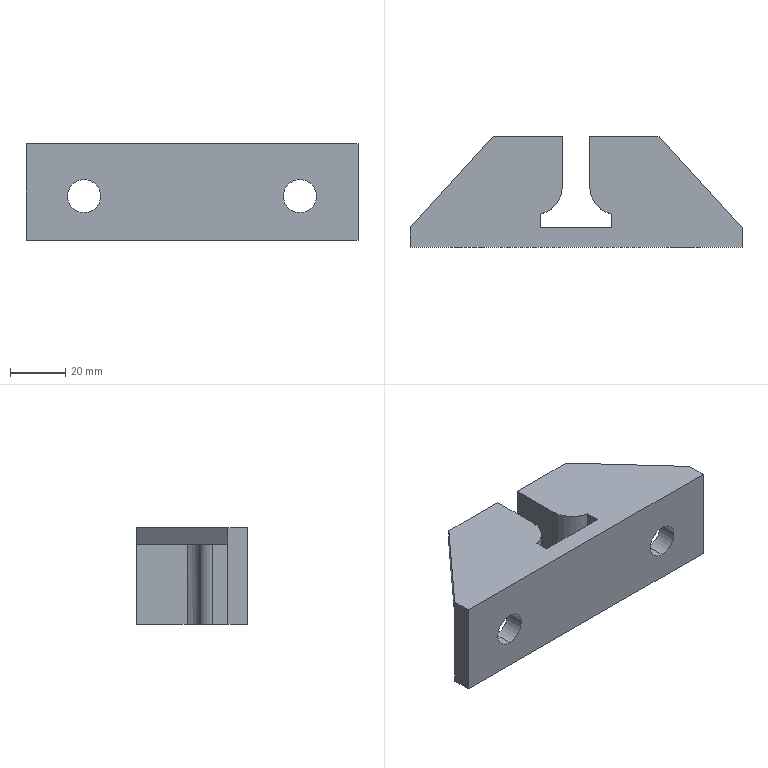Part | SolidWorks | features ICE 3, Fillet 2, MirrorPattern 2, Extrusion 1 | 1 solid | 32 faces | box 120 x 40 x 35 mm | volume 52086 mm3 | plane 22 | cylinder 8 | spline 2 | commonest cylinder face diameters 12 x4 10 x2 20 x2
STEP:
#1=CARTESIAN_POINT('',(39.,0.,-4.638));
#2=VERTEX_POINT('',#1);
#3=CARTESIAN_POINT('',(39.,0.,-16.638));
#4=VERTEX_POINT('',#3);
#5=CARTESIAN_POINT('',(39.,0.,-10.638));
#6=DIRECTION('',(0.,-1.,0.));
#7=DIRECTION('',(0.,0.,1.));
#8=AXIS2_PLACEMENT_3D('',#5,#6,#7);
#9=CIRCLE('',#8,6.);
#10=EDGE_CURVE('',#2,#4,#9,.T.);
#11=ORIENTED_EDGE('',*,*,#10,.T.);
#12=CARTESIAN_POINT('',(39.,7.,-16.638));
#13=VERTEX_POINT('',#12);
#14=CARTESIAN_POINT('',(39.,-3.,-16.638));
#15=DIRECTION('',(0.,1.,0.));
#16=VECTOR('',#15,1000.);
#17=LINE('',#14,#16);
#18=EDGE_CURVE('',#4,#13,#17,.T.);
#19=ORIENTED_EDGE('',*,*,#18,.T.);
#20=CARTESIAN_POINT('',(39.,7.,-4.638));
#21=VERTEX_POINT('',#20);
#22=CARTESIAN_POINT('',(39.,7.,-10.638));
#23=DIRECTION('',(0.,-1.,0.));
#24=DIRECTION('',(0.,0.,1.));
#25=AXIS2_PLACEMENT_3D('',#22,#23,#24);
#26=CIRCLE('',#25,6.);
#27=EDGE_CURVE('',#21,#13,#26,.T.);
#28=ORIENTED_EDGE('',*,*,#27,.F.);
#29=CARTESIAN_POINT('',(39.,-3.,-4.638));
#30=DIRECTION('',(0.,1.,0.));
#31=VECTOR('',#30,1000.);
#32=LINE('',#29,#31);
#33=EDGE_CURVE('',#2,#21,#32,.T.);
#34=ORIENTED_EDGE('',*,*,#33,.F.);
#35=EDGE_LOOP('',(#11,#19,#28,#34));
#36=FACE_OUTER_BOUND('',#35,.T.);
#37=CARTESIAN_POINT('',(39.,-3.,-10.638));
#38=DIRECTION('',(0.,1.,0.));
#39=DIRECTION('',(0.,0.,1.));
#40=AXIS2_PLACEMENT_3D('',#37,#38,#39);
#41=CYLINDRICAL_SURFACE('',#40,6.);
#42=ADVANCED_FACE('',(#36),#41,.F.);
#43=CARTESIAN_POINT('',(-39.,0.,-16.638));
#44=VERTEX_POINT('',#43);
#45=CARTESIAN_POINT('',(-39.,0.,-4.638));
#46=VERTEX_POINT('',#45);
#47=CARTESIAN_POINT('',(-39.,0.,-10.638));
#48=DIRECTION('',(0.,1.,0.));
#49=DIRECTION('',(0.,0.,1.));
#50=AXIS2_PLACEMENT_3D('',#47,#48,#49);
#51=CIRCLE('',#50,6.);
#52=EDGE_CURVE('',#44,#46,#51,.T.);
#53=ORIENTED_EDGE('',*,*,#52,.F.);
#54=CARTESIAN_POINT('',(-39.,7.,-16.638));
#55=VERTEX_POINT('',#54);
#56=CARTESIAN_POINT('',(-39.,-3.,-16.638));
#57=DIRECTION('',(0.,1.,0.));
#58=VECTOR('',#57,1000.);
#59=LINE('',#56,#58);
#60=EDGE_CURVE('',#44,#55,#59,.T.);
#61=ORIENTED_EDGE('',*,*,#60,.T.);
#62=CARTESIAN_POINT('',(-39.,7.,-4.638));
#63=VERTEX_POINT('',#62);
#64=CARTESIAN_POINT('',(-39.,7.,-10.638));
#65=DIRECTION('',(0.,1.,0.));
#66=DIRECTION('',(0.,0.,1.));
#67=AXIS2_PLACEMENT_3D('',#64,#65,#66);
#68=CIRCLE('',#67,6.);
#69=EDGE_CURVE('',#55,#63,#68,.T.);
#70=ORIENTED_EDGE('',*,*,#69,.T.);
#71=CARTESIAN_POINT('',(-39.,-3.,-4.638));
#72=DIRECTION('',(0.,1.,0.));
#73=VECTOR('',#72,1000.);
#74=LINE('',#71,#73);
#75=EDGE_CURVE('',#46,#63,#74,.T.);
#76=ORIENTED_EDGE('',*,*,#75,.F.);
#77=EDGE_LOOP('',(#53,#61,#70,#76));
#78=FACE_OUTER_BOUND('',#77,.T.);
#79=CARTESIAN_POINT('',(-39.,-3.,-10.638));
#80=DIRECTION('',(0.,1.,0.));
#81=DIRECTION('',(0.,0.,1.));
#82=AXIS2_PLACEMENT_3D('',#79,#80,#81);
#83=CYLINDRICAL_SURFACE('',#82,6.);
#84=ADVANCED_FACE('',(#78),#83,.F.);
#85=CARTESIAN_POINT('',(17.,7.,-26.638));
#86=VERTEX_POINT('',#85);
#87=CARTESIAN_POINT('',(17.,7.,2.362));
#88=VERTEX_POINT('',#87);
#89=CARTESIAN_POINT('',(17.,7.,-61.752));
#90=DIRECTION('',(0.,0.,1.));
#91=VECTOR('',#90,1000.);
#92=LINE('',#89,#91);
#93=EDGE_CURVE('',#86,#88,#92,.T.);
#94=ORIENTED_EDGE('',*,*,#93,.T.);
#95=CARTESIAN_POINT('',(60.,7.,2.362));
#96=VERTEX_POINT('',#95);
#97=CARTESIAN_POINT('',(13.,7.,2.362));
#98=DIRECTION('',(-1.,0.,0.));
#99=VECTOR('',#98,1000.);
#100=LINE('',#97,#99);
#101=EDGE_CURVE('',#96,#88,#100,.T.);
#102=ORIENTED_EDGE('',*,*,#101,.F.);
#103=CARTESIAN_POINT('',(60.,7.,-26.638));
#104=VERTEX_POINT('',#103);
#105=CARTESIAN_POINT('',(60.,7.,-26.638));
#106=DIRECTION('',(0.,0.,-1.));
#107=VECTOR('',#106,1000.);
#108=LINE('',#105,#107);
#109=EDGE_CURVE('',#96,#104,#108,.T.);
#110=ORIENTED_EDGE('',*,*,#109,.T.);
#111=CARTESIAN_POINT('',(-60.,7.,-26.638));
#112=DIRECTION('',(-1.,0.,0.));
#113=VECTOR('',#112,1000.);
#114=LINE('',#111,#113);
#115=EDGE_CURVE('',#104,#86,#114,.T.);
#116=ORIENTED_EDGE('',*,*,#115,.T.);
#117=EDGE_LOOP('',(#94,#102,#110,#116));
#118=FACE_OUTER_BOUND('',#117,.T.);
#119=ORIENTED_EDGE('',*,*,#27,.T.);
#120=CARTESIAN_POINT('',(39.,7.,-10.638));
#121=DIRECTION('',(0.,-1.,0.));
#122=DIRECTION('',(0.,0.,1.));
#123=AXIS2_PLACEMENT_3D('',#120,#121,#122);
#124=CIRCLE('',#123,6.);
#125=EDGE_CURVE('',#13,#21,#124,.T.);
#126=ORIENTED_EDGE('',*,*,#125,.T.);
#127=EDGE_LOOP('',(#119,#126));
#128=FACE_BOUND('',#127,.T.);
#129=CARTESIAN_POINT('',(0.,7.,0.));
#130=DIRECTION('',(0.,1.,0.));
#131=DIRECTION('',(0.,0.,1.));
#132=AXIS2_PLACEMENT_3D('',#129,#130,#131);
#133=PLANE('',#132);
#134=ADVANCED_FACE('',(#118,#128),#133,.T.);
#135=CARTESIAN_POINT('',(-60.,0.,-26.638));
#136=VERTEX_POINT('',#135);
#137=CARTESIAN_POINT('',(-60.,0.,8.362));
#138=VERTEX_POINT('',#137);
#139=CARTESIAN_POINT('',(-60.,0.,-26.638));
#140=DIRECTION('',(0.,0.,1.));
#141=VECTOR('',#140,1000.);
#142=LINE('',#139,#141);
#143=EDGE_CURVE('',#136,#138,#142,.T.);
#144=ORIENTED_EDGE('',*,*,#143,.F.);
#145=CARTESIAN_POINT('',(60.,0.,-26.638));
#146=VERTEX_POINT('',#145);
#147=CARTESIAN_POINT('',(-60.,0.,-26.638));
#148=DIRECTION('',(-1.,0.,0.));
#149=VECTOR('',#148,1000.);
#150=LINE('',#147,#149);
#151=EDGE_CURVE('',#146,#136,#150,.T.);
#152=ORIENTED_EDGE('',*,*,#151,.F.);
#153=CARTESIAN_POINT('',(60.,0.,8.362));
#154=VERTEX_POINT('',#153);
#155=CARTESIAN_POINT('',(60.,0.,-26.638));
#156=DIRECTION('',(0.,0.,-1.));
#157=VECTOR('',#156,1000.);
#158=LINE('',#155,#157);
#159=EDGE_CURVE('',#154,#146,#158,.T.);
#160=ORIENTED_EDGE('',*,*,#159,.F.);
#161=CARTESIAN_POINT('',(-60.,0.,8.362));
#162=DIRECTION('',(1.,0.,0.));
#163=VECTOR('',#162,1000.);
#164=LINE('',#161,#163);
#165=EDGE_CURVE('',#138,#154,#164,.T.);
#166=ORIENTED_EDGE('',*,*,#165,.F.);
#167=EDGE_LOOP('',(#144,#152,#160,#166));
#168=FACE_OUTER_BOUND('',#167,.T.);
#169=CARTESIAN_POINT('',(-39.,0.,-10.638));
#170=DIRECTION('',(0.,1.,0.));
#171=DIRECTION('',(0.,0.,1.));
#172=AXIS2_PLACEMENT_3D('',#169,#170,#171);
#173=CIRCLE('',#172,6.);
#174=EDGE_CURVE('',#46,#44,#173,.T.);
#175=ORIENTED_EDGE('',*,*,#174,.T.);
#176=ORIENTED_EDGE('',*,*,#52,.T.);
#177=EDGE_LOOP('',(#175,#176));
#178=FACE_BOUND('',#177,.T.);
#179=ORIENTED_EDGE('',*,*,#10,.F.);
#180=CARTESIAN_POINT('',(39.,0.,-10.638));
#181=DIRECTION('',(0.,-1.,0.));
#182=DIRECTION('',(0.,0.,1.));
#183=AXIS2_PLACEMENT_3D('',#180,#181,#182);
#184=CIRCLE('',#183,6.);
#185=EDGE_CURVE('',#4,#2,#184,.T.);
#186=ORIENTED_EDGE('',*,*,#185,.F.);
#187=EDGE_LOOP('',(#179,#186));
#188=FACE_BOUND('',#187,.T.);
#189=CARTESIAN_POINT('',(0.,0.,0.));
#190=DIRECTION('',(0.,1.,0.));
#191=DIRECTION('',(0.,0.,1.));
#192=AXIS2_PLACEMENT_3D('',#189,#190,#191);
#193=PLANE('',#192);
#194=ADVANCED_FACE('',(#168,#178,#188),#193,.F.);
#195=CARTESIAN_POINT('',(13.,7.,-26.638));
#196=VERTEX_POINT('',#195);
#197=CARTESIAN_POINT('',(13.,7.,8.362));
#198=VERTEX_POINT('',#197);
#199=CARTESIAN_POINT('',(13.,7.,2.362));
#200=DIRECTION('',(0.,0.,1.));
#201=VECTOR('',#200,1000.);
#202=LINE('',#199,#201);
#203=EDGE_CURVE('',#196,#198,#202,.T.);
#204=ORIENTED_EDGE('',*,*,#203,.F.);
#205=CARTESIAN_POINT('',(-13.,7.,-26.638));
#206=VERTEX_POINT('',#205);
#207=CARTESIAN_POINT('',(-60.,7.,-26.638));
#208=DIRECTION('',(-1.,0.,0.));
#209=VECTOR('',#208,1000.);
#210=LINE('',#207,#209);
#211=EDGE_CURVE('',#196,#206,#210,.T.);
#212=ORIENTED_EDGE('',*,*,#211,.T.);
#213=CARTESIAN_POINT('',(-13.,7.,8.362));
#214=VERTEX_POINT('',#213);
#215=CARTESIAN_POINT('',(-13.,7.,2.362));
#216=DIRECTION('',(0.,0.,1.));
#217=VECTOR('',#216,1000.);
#218=LINE('',#215,#217);
#219=EDGE_CURVE('',#206,#214,#218,.T.);
#220=ORIENTED_EDGE('',*,*,#219,.T.);
#221=CARTESIAN_POINT('',(-60.,7.,8.362));
#222=DIRECTION('',(1.,0.,0.));
#223=VECTOR('',#222,1000.);
#224=LINE('',#221,#223);
#225=EDGE_CURVE('',#214,#198,#224,.T.);
#226=ORIENTED_EDGE('',*,*,#225,.T.);
#227=EDGE_LOOP('',(#204,#212,#220,#226));
#228=FACE_OUTER_BOUND('',#227,.T.);
#229=CARTESIAN_POINT('',(0.,7.,0.));
#230=DIRECTION('',(0.,1.,0.));
#231=DIRECTION('',(0.,0.,1.));
#232=AXIS2_PLACEMENT_3D('',#229,#230,#231);
#233=PLANE('',#232);
#234=ADVANCED_FACE('',(#228),#233,.T.);
#235=CARTESIAN_POINT('',(-39.,7.,-10.638));
#236=DIRECTION('',(0.,1.,0.));
#237=DIRECTION('',(0.,0.,1.));
#238=AXIS2_PLACEMENT_3D('',#235,#236,#237);
#239=CIRCLE('',#238,6.);
#240=EDGE_CURVE('',#63,#55,#239,.T.);
#241=ORIENTED_EDGE('',*,*,#240,.F.);
#242=ORIENTED_EDGE('',*,*,#69,.F.);
#243=EDGE_LOOP('',(#241,#242));
#244=FACE_BOUND('',#243,.T.);
#245=CARTESIAN_POINT('',(-60.,7.,2.362));
#246=VERTEX_POINT('',#245);
#247=CARTESIAN_POINT('',(-17.,7.,2.362));
#248=VERTEX_POINT('',#247);
#249=CARTESIAN_POINT('',(-13.,7.,2.362));
#250=DIRECTION('',(1.,0.,0.));
#251=VECTOR('',#250,1000.);
#252=LINE('',#249,#251);
#253=EDGE_CURVE('',#246,#248,#252,.T.);
#254=ORIENTED_EDGE('',*,*,#253,.T.);
#255=CARTESIAN_POINT('',(-17.,7.,-26.638));
#256=VERTEX_POINT('',#255);
#257=CARTESIAN_POINT('',(-17.,7.,-61.752));
#258=DIRECTION('',(0.,0.,1.));
#259=VECTOR('',#258,1000.);
#260=LINE('',#257,#259);
#261=EDGE_CURVE('',#256,#248,#260,.T.);
#262=ORIENTED_EDGE('',*,*,#261,.F.);
#263=CARTESIAN_POINT('',(-60.,7.,-26.638));
#264=VERTEX_POINT('',#263);
#265=CARTESIAN_POINT('',(-60.,7.,-26.638));
#266=DIRECTION('',(-1.,0.,0.));
#267=VECTOR('',#266,1000.);
#268=LINE('',#265,#267);
#269=EDGE_CURVE('',#256,#264,#268,.T.);
#270=ORIENTED_EDGE('',*,*,#269,.T.);
#271=CARTESIAN_POINT('',(-60.,7.,-26.638));
#272=DIRECTION('',(0.,0.,1.));
#273=VECTOR('',#272,1000.);
#274=LINE('',#271,#273);
#275=EDGE_CURVE('',#264,#246,#274,.T.);
#276=ORIENTED_EDGE('',*,*,#275,.T.);
#277=EDGE_LOOP('',(#254,#262,#270,#276));
#278=FACE_OUTER_BOUND('',#277,.T.);
#279=CARTESIAN_POINT('',(0.,7.,0.));
#280=DIRECTION('',(0.,1.,0.));
#281=DIRECTION('',(0.,0.,1.));
#282=AXIS2_PLACEMENT_3D('',#279,#280,#281);
#283=PLANE('',#282);
#284=ADVANCED_FACE('',(#244,#278),#283,.T.);
#285=CARTESIAN_POINT('',(-9.,21.798,2.362));
#286=VERTEX_POINT('',#285);
#287=CARTESIAN_POINT('',(-9.,40.,2.362));
#288=VERTEX_POINT('',#287);
#289=CARTESIAN_POINT('',(-9.,21.798,2.362));
#290=DIRECTION('',(0.,1.,0.));
#291=VECTOR('',#290,1000.);
#292=LINE('',#289,#291);
#293=EDGE_CURVE('',#286,#288,#292,.T.);
#294=ORIENTED_EDGE('',*,*,#293,.F.);
#295=CARTESIAN_POINT('',(-13.534,17.332,2.362));
#296=VERTEX_POINT('',#295);
#297=CARTESIAN_POINT('',(-13.534,17.332,2.362));
#298=CARTESIAN_POINT('',(-10.568,18.288,2.362));
#299=CARTESIAN_POINT('',(-9.,21.798,2.362));
#300=B_SPLINE_CURVE_WITH_KNOTS('',2,(#297,#298,#299),.UNSPECIFIED.,.F.,.F.,(3,3),(0.3423,1.),.UNSPECIFIED.);
#301=EDGE_CURVE('',#296,#286,#300,.T.);
#302=ORIENTED_EDGE('',*,*,#301,.F.);
#303=CARTESIAN_POINT('',(-17.,12.573,2.362));
#304=VERTEX_POINT('',#303);
#305=CARTESIAN_POINT('',(-12.,12.573,2.362));
#306=DIRECTION('',(0.,0.,1.));
#307=DIRECTION('',(1.,0.,0.));
#308=AXIS2_PLACEMENT_3D('',#305,#306,#307);
#309=CIRCLE('',#308,5.);
#310=EDGE_CURVE('',#296,#304,#309,.T.);
#311=ORIENTED_EDGE('',*,*,#310,.T.);
#312=CARTESIAN_POINT('',(-17.,15.,2.362));
#313=DIRECTION('',(0.,1.,0.));
#314=VECTOR('',#313,1000.);
#315=LINE('',#312,#314);
#316=EDGE_CURVE('',#248,#304,#315,.T.);
#317=ORIENTED_EDGE('',*,*,#316,.F.);
#318=ORIENTED_EDGE('',*,*,#253,.F.);
#319=CARTESIAN_POINT('',(-30.,40.,2.362));
#320=VERTEX_POINT('',#319);
#321=CARTESIAN_POINT('',(-60.,7.,2.362));
#322=DIRECTION('',(-0.6727,-0.7399,0.));
#323=VECTOR('',#322,1000.);
#324=LINE('',#321,#323);
#325=EDGE_CURVE('',#320,#246,#324,.T.);
#326=ORIENTED_EDGE('',*,*,#325,.F.);
#327=CARTESIAN_POINT('',(-30.,40.,2.362));
#328=DIRECTION('',(-1.,0.,0.));
#329=VECTOR('',#328,1000.);
#330=LINE('',#327,#329);
#331=EDGE_CURVE('',#288,#320,#330,.T.);
#332=ORIENTED_EDGE('',*,*,#331,.F.);
#333=EDGE_LOOP('',(#294,#302,#311,#317,#318,#326,#332));
#334=FACE_OUTER_BOUND('',#333,.T.);
#335=CARTESIAN_POINT('',(0.,0.,2.362));
#336=DIRECTION('',(0.,0.,1.));
#337=DIRECTION('',(1.,0.,0.));
#338=AXIS2_PLACEMENT_3D('',#335,#336,#337);
#339=PLANE('',#338);
#340=ADVANCED_FACE('',(#334),#339,.F.);
#341=ORIENTED_EDGE('',*,*,#143,.T.);
#342=CARTESIAN_POINT('',(-60.,7.,8.362));
#343=VERTEX_POINT('',#342);
#344=CARTESIAN_POINT('',(-60.,7.,8.362));
#345=DIRECTION('',(0.,-1.,0.));
#346=VECTOR('',#345,1000.);
#347=LINE('',#344,#346);
#348=EDGE_CURVE('',#343,#138,#347,.T.);
#349=ORIENTED_EDGE('',*,*,#348,.F.);
#350=CARTESIAN_POINT('',(-60.,7.,2.362));
#351=DIRECTION('',(0.,0.,1.));
#352=VECTOR('',#351,1000.);
#353=LINE('',#350,#352);
#354=EDGE_CURVE('',#246,#343,#353,.T.);
#355=ORIENTED_EDGE('',*,*,#354,.F.);
#356=ORIENTED_EDGE('',*,*,#275,.F.);
#357=CARTESIAN_POINT('',(-60.,7.,-26.638));
#358=DIRECTION('',(0.,-1.,0.));
#359=VECTOR('',#358,1000.);
#360=LINE('',#357,#359);
#361=EDGE_CURVE('',#264,#136,#360,.T.);
#362=ORIENTED_EDGE('',*,*,#361,.T.);
#363=EDGE_LOOP('',(#341,#349,#355,#356,#362));
#364=FACE_OUTER_BOUND('',#363,.T.);
#365=CARTESIAN_POINT('',(-60.,7.,-26.638));
#366=DIRECTION('',(1.,0.,0.));
#367=DIRECTION('',(0.,0.,-1.));
#368=AXIS2_PLACEMENT_3D('',#365,#366,#367);
#369=PLANE('',#368);
#370=ADVANCED_FACE('',(#364),#369,.F.);
#371=CARTESIAN_POINT('',(5.,21.798,8.362));
#372=VERTEX_POINT('',#371);
#373=CARTESIAN_POINT('',(5.,40.,8.362));
#374=VERTEX_POINT('',#373);
#375=CARTESIAN_POINT('',(5.,40.,8.362));
#376=DIRECTION('',(0.,1.,0.));
#377=VECTOR('',#376,1000.);
#378=LINE('',#375,#377);
#379=EDGE_CURVE('',#372,#374,#378,.T.);
#380=ORIENTED_EDGE('',*,*,#379,.F.);
#381=CARTESIAN_POINT('',(13.,12.,8.362));
#382=VERTEX_POINT('',#381);
#383=CARTESIAN_POINT('',(15.,21.798,8.362));
#384=DIRECTION('',(0.,0.,1.));
#385=DIRECTION('',(-1.,0.,0.));
#386=AXIS2_PLACEMENT_3D('',#383,#384,#385);
#387=CIRCLE('',#386,10.);
#388=EDGE_CURVE('',#372,#382,#387,.T.);
#389=ORIENTED_EDGE('',*,*,#388,.T.);
#390=CARTESIAN_POINT('',(13.,12.,8.362));
#391=DIRECTION('',(0.,1.,0.));
#392=VECTOR('',#391,1000.);
#393=LINE('',#390,#392);
#394=EDGE_CURVE('',#198,#382,#393,.T.);
#395=ORIENTED_EDGE('',*,*,#394,.F.);
#396=ORIENTED_EDGE('',*,*,#225,.F.);
#397=CARTESIAN_POINT('',(-13.,12.,8.362));
#398=VERTEX_POINT('',#397);
#399=CARTESIAN_POINT('',(-13.,12.,8.362));
#400=DIRECTION('',(0.,1.,0.));
#401=VECTOR('',#400,1000.);
#402=LINE('',#399,#401);
#403=EDGE_CURVE('',#214,#398,#402,.T.);
#404=ORIENTED_EDGE('',*,*,#403,.T.);
#405=CARTESIAN_POINT('',(-5.,21.798,8.362));
#406=VERTEX_POINT('',#405);
#407=CARTESIAN_POINT('',(-15.,21.798,8.362));
#408=DIRECTION('',(0.,0.,1.));
#409=DIRECTION('',(-1.,0.,0.));
#410=AXIS2_PLACEMENT_3D('',#407,#408,#409);
#411=CIRCLE('',#410,10.);
#412=EDGE_CURVE('',#398,#406,#411,.T.);
#413=ORIENTED_EDGE('',*,*,#412,.T.);
#414=CARTESIAN_POINT('',(-5.,40.,8.362));
#415=VERTEX_POINT('',#414);
#416=CARTESIAN_POINT('',(-5.,40.,8.362));
#417=DIRECTION('',(0.,1.,0.));
#418=VECTOR('',#417,1000.);
#419=LINE('',#416,#418);
#420=EDGE_CURVE('',#406,#415,#419,.T.);
#421=ORIENTED_EDGE('',*,*,#420,.T.);
#422=CARTESIAN_POINT('',(-30.,40.,8.362));
#423=VERTEX_POINT('',#422);
#424=CARTESIAN_POINT('',(-30.,40.,8.362));
#425=DIRECTION('',(-1.,0.,0.));
#426=VECTOR('',#425,1000.);
#427=LINE('',#424,#426);
#428=EDGE_CURVE('',#415,#423,#427,.T.);
#429=ORIENTED_EDGE('',*,*,#428,.T.);
#430=CARTESIAN_POINT('',(-60.,7.,8.362));
#431=DIRECTION('',(-0.6727,-0.7399,0.));
#432=VECTOR('',#431,1000.);
#433=LINE('',#430,#432);
#434=EDGE_CURVE('',#423,#343,#433,.T.);
#435=ORIENTED_EDGE('',*,*,#434,.T.);
#436=ORIENTED_EDGE('',*,*,#348,.T.);
#437=ORIENTED_EDGE('',*,*,#165,.T.);
#438=CARTESIAN_POINT('',(60.,7.,8.362));
#439=VERTEX_POINT('',#438);
#440=CARTESIAN_POINT('',(60.,7.,8.362));
#441=DIRECTION('',(0.,-1.,0.));
#442=VECTOR('',#441,1000.);
#443=LINE('',#440,#442);
#444=EDGE_CURVE('',#439,#154,#443,.T.);
#445=ORIENTED_EDGE('',*,*,#444,.F.);
#446=CARTESIAN_POINT('',(30.,40.,8.362));
#447=VERTEX_POINT('',#446);
#448=CARTESIAN_POINT('',(60.,7.,8.362));
#449=DIRECTION('',(0.6727,-0.7399,0.));
#450=VECTOR('',#449,1000.);
#451=LINE('',#448,#450);
#452=EDGE_CURVE('',#447,#439,#451,.T.);
#453=ORIENTED_EDGE('',*,*,#452,.F.);
#454=CARTESIAN_POINT('',(30.,40.,8.362));
#455=DIRECTION('',(1.,0.,0.));
#456=VECTOR('',#455,1000.);
#457=LINE('',#454,#456);
#458=EDGE_CURVE('',#374,#447,#457,.T.);
#459=ORIENTED_EDGE('',*,*,#458,.F.);
#460=EDGE_LOOP('',(#380,#389,#395,#396,#404,#413,#421,#429,#435,#436,#437,#445,#453,#459));
#461=FACE_OUTER_BOUND('',#460,.T.);
#462=CARTESIAN_POINT('',(-60.,7.,8.362));
#463=DIRECTION('',(0.,0.,-1.));
#464=DIRECTION('',(-1.,0.,0.));
#465=AXIS2_PLACEMENT_3D('',#462,#463,#464);
#466=PLANE('',#465);
#467=ADVANCED_FACE('',(#461),#466,.F.);
#468=ORIENTED_EDGE('',*,*,#159,.T.);
#469=CARTESIAN_POINT('',(60.,7.,-26.638));
#470=DIRECTION('',(0.,-1.,0.));
#471=VECTOR('',#470,1000.);
#472=LINE('',#469,#471);
#473=EDGE_CURVE('',#104,#146,#472,.T.);
#474=ORIENTED_EDGE('',*,*,#473,.F.);
#475=ORIENTED_EDGE('',*,*,#109,.F.);
#476=CARTESIAN_POINT('',(60.,7.,-26.638));
#477=DIRECTION('',(0.,0.,-1.));
#478=VECTOR('',#477,1000.);
#479=LINE('',#476,#478);
#480=EDGE_CURVE('',#439,#96,#479,.T.);
#481=ORIENTED_EDGE('',*,*,#480,.F.);
#482=ORIENTED_EDGE('',*,*,#444,.T.);
#483=EDGE_LOOP('',(#468,#474,#475,#481,#482));
#484=FACE_OUTER_BOUND('',#483,.T.);
#485=CARTESIAN_POINT('',(60.,7.,-26.638));
#486=DIRECTION('',(-1.,0.,0.));
#487=DIRECTION('',(0.,0.,1.));
#488=AXIS2_PLACEMENT_3D('',#485,#486,#487);
#489=PLANE('',#488);
#490=ADVANCED_FACE('',(#484),#489,.F.);
#491=CARTESIAN_POINT('',(-17.,12.573,-26.638));
#492=VERTEX_POINT('',#491);
#493=CARTESIAN_POINT('',(-17.,15.,-26.638));
#494=DIRECTION('',(0.,-1.,0.));
#495=VECTOR('',#494,1000.);
#496=LINE('',#493,#495);
#497=EDGE_CURVE('',#492,#256,#496,.T.);
#498=ORIENTED_EDGE('',*,*,#497,.F.);
#499=CARTESIAN_POINT('',(-13.534,17.332,-26.638));
#500=VERTEX_POINT('',#499);
#501=CARTESIAN_POINT('',(-12.,12.573,-26.638));
#502=DIRECTION('',(0.,0.,-1.));
#503=DIRECTION('',(1.,0.,0.));
#504=AXIS2_PLACEMENT_3D('',#501,#502,#503);
#505=CIRCLE('',#504,5.);
#506=EDGE_CURVE('',#492,#500,#505,.T.);
#507=ORIENTED_EDGE('',*,*,#506,.T.);
#508=CARTESIAN_POINT('',(-9.,21.798,-26.638));
#509=VERTEX_POINT('',#508);
#510=CARTESIAN_POINT('',(-9.,21.798,-26.638));
#511=CARTESIAN_POINT('',(-10.568,18.288,-26.638));
#512=CARTESIAN_POINT('',(-13.534,17.332,-26.638));
#513=B_SPLINE_CURVE_WITH_KNOTS('',2,(#510,#511,#512),.UNSPECIFIED.,.F.,.F.,(3,3),(0.,0.6577),.UNSPECIFIED.);
#514=EDGE_CURVE('',#509,#500,#513,.T.);
#515=ORIENTED_EDGE('',*,*,#514,.F.);
#516=CARTESIAN_POINT('',(-9.,40.,-26.638));
#517=VERTEX_POINT('',#516);
#518=CARTESIAN_POINT('',(-9.,21.798,-26.638));
#519=DIRECTION('',(0.,-1.,0.));
#520=VECTOR('',#519,1000.);
#521=LINE('',#518,#520);
#522=EDGE_CURVE('',#517,#509,#521,.T.);
#523=ORIENTED_EDGE('',*,*,#522,.F.);
#524=CARTESIAN_POINT('',(-5.,40.,-26.638));
#525=VERTEX_POINT('',#524);
#526=CARTESIAN_POINT('',(-5.,40.,-26.638));
#527=DIRECTION('',(-1.,0.,0.));
#528=VECTOR('',#527,1000.);
#529=LINE('',#526,#528);
#530=EDGE_CURVE('',#525,#517,#529,.T.);
#531=ORIENTED_EDGE('',*,*,#530,.F.);
#532=CARTESIAN_POINT('',(-5.,21.798,-26.638));
#533=VERTEX_POINT('',#532);
#534=CARTESIAN_POINT('',(-5.,21.798,-26.638));
#535=DIRECTION('',(0.,1.,0.));
#536=VECTOR('',#535,1000.);
#537=LINE('',#534,#536);
#538=EDGE_CURVE('',#533,#525,#537,.T.);
#539=ORIENTED_EDGE('',*,*,#538,.F.);
#540=CARTESIAN_POINT('',(-13.,12.,-26.638));
#541=VERTEX_POINT('',#540);
#542=CARTESIAN_POINT('',(-15.,21.798,-26.638));
#543=DIRECTION('',(0.,0.,1.));
#544=DIRECTION('',(1.,0.,0.));
#545=AXIS2_PLACEMENT_3D('',#542,#543,#544);
#546=CIRCLE('',#545,10.);
#547=EDGE_CURVE('',#541,#533,#546,.T.);
#548=ORIENTED_EDGE('',*,*,#547,.F.);
#549=CARTESIAN_POINT('',(-13.,7.,-26.638));
#550=DIRECTION('',(0.,1.,0.));
#551=VECTOR('',#550,1000.);
#552=LINE('',#549,#551);
#553=EDGE_CURVE('',#206,#541,#552,.T.);
#554=ORIENTED_EDGE('',*,*,#553,.F.);
#555=ORIENTED_EDGE('',*,*,#211,.F.);
#556=CARTESIAN_POINT('',(13.,12.,-26.638));
#557=VERTEX_POINT('',#556);
#558=CARTESIAN_POINT('',(13.,7.,-26.638));
#559=DIRECTION('',(0.,1.,0.));
#560=VECTOR('',#559,1000.);
#561=LINE('',#558,#560);
#562=EDGE_CURVE('',#196,#557,#561,.T.);
#563=ORIENTED_EDGE('',*,*,#562,.T.);
#564=CARTESIAN_POINT('',(5.,21.798,-26.638));
#565=VERTEX_POINT('',#564);
#566=CARTESIAN_POINT('',(15.,21.798,-26.638));
#567=DIRECTION('',(0.,0.,-1.));
#568=DIRECTION('',(1.,0.,0.));
#569=AXIS2_PLACEMENT_3D('',#566,#567,#568);
#570=CIRCLE('',#569,10.);
#571=EDGE_CURVE('',#557,#565,#570,.T.);
#572=ORIENTED_EDGE('',*,*,#571,.T.);
#573=CARTESIAN_POINT('',(5.,40.,-26.638));
#574=VERTEX_POINT('',#573);
#575=CARTESIAN_POINT('',(5.,21.798,-26.638));
#576=DIRECTION('',(0.,1.,0.));
#577=VECTOR('',#576,1000.);
#578=LINE('',#575,#577);
#579=EDGE_CURVE('',#565,#574,#578,.T.);
#580=ORIENTED_EDGE('',*,*,#579,.T.);
#581=CARTESIAN_POINT('',(9.,40.,-26.638));
#582=VERTEX_POINT('',#581);
#583=CARTESIAN_POINT('',(5.,40.,-26.638));
#584=DIRECTION('',(1.,0.,0.));
#585=VECTOR('',#584,1000.);
#586=LINE('',#583,#585);
#587=EDGE_CURVE('',#574,#582,#586,.T.);
#588=ORIENTED_EDGE('',*,*,#587,.T.);
#589=CARTESIAN_POINT('',(9.,21.798,-26.638));
#590=VERTEX_POINT('',#589);
#591=CARTESIAN_POINT('',(9.,21.798,-26.638));
#592=DIRECTION('',(0.,-1.,0.));
#593=VECTOR('',#592,1000.);
#594=LINE('',#591,#593);
#595=EDGE_CURVE('',#582,#590,#594,.T.);
#596=ORIENTED_EDGE('',*,*,#595,.T.);
#597=CARTESIAN_POINT('',(13.534,17.332,-26.638));
#598=VERTEX_POINT('',#597);
#599=CARTESIAN_POINT('',(9.,21.798,-26.638));
#600=CARTESIAN_POINT('',(10.568,18.288,-26.638));
#601=CARTESIAN_POINT('',(13.534,17.332,-26.638));
#602=B_SPLINE_CURVE_WITH_KNOTS('',2,(#599,#600,#601),.UNSPECIFIED.,.F.,.F.,(3,3),(0.,0.6577),.UNSPECIFIED.);
#603=EDGE_CURVE('',#590,#598,#602,.T.);
#604=ORIENTED_EDGE('',*,*,#603,.T.);
#605=CARTESIAN_POINT('',(17.,12.573,-26.638));
#606=VERTEX_POINT('',#605);
#607=CARTESIAN_POINT('',(12.,12.573,-26.638));
#608=DIRECTION('',(0.,0.,-1.));
#609=DIRECTION('',(1.,0.,0.));
#610=AXIS2_PLACEMENT_3D('',#607,#608,#609);
#611=CIRCLE('',#610,5.);
#612=EDGE_CURVE('',#598,#606,#611,.T.);
#613=ORIENTED_EDGE('',*,*,#612,.T.);
#614=CARTESIAN_POINT('',(17.,7.,-26.638));
#615=DIRECTION('',(0.,-1.,0.));
#616=VECTOR('',#615,1000.);
#617=LINE('',#614,#616);
#618=EDGE_CURVE('',#606,#86,#617,.T.);
#619=ORIENTED_EDGE('',*,*,#618,.T.);
#620=ORIENTED_EDGE('',*,*,#115,.F.);
#621=ORIENTED_EDGE('',*,*,#473,.T.);
#622=ORIENTED_EDGE('',*,*,#151,.T.);
#623=ORIENTED_EDGE('',*,*,#361,.F.);
#624=ORIENTED_EDGE('',*,*,#269,.F.);
#625=EDGE_LOOP('',(#498,#507,#515,#523,#531,#539,#548,#554,#555,#563,#572,#580,#588,#596,#604,#613,#619,#620,#621,#622,#623,#624));
#626=FACE_OUTER_BOUND('',#625,.T.);
#627=CARTESIAN_POINT('',(-60.,7.,-26.638));
#628=DIRECTION('',(0.,0.,1.));
#629=DIRECTION('',(1.,0.,0.));
#630=AXIS2_PLACEMENT_3D('',#627,#628,#629);
#631=PLANE('',#630);
#632=ADVANCED_FACE('',(#626),#631,.F.);
#633=ORIENTED_EDGE('',*,*,#434,.F.);
#634=CARTESIAN_POINT('',(-30.,40.,2.362));
#635=DIRECTION('',(0.,0.,1.));
#636=VECTOR('',#635,1000.);
#637=LINE('',#634,#636);
#638=EDGE_CURVE('',#320,#423,#637,.T.);
#639=ORIENTED_EDGE('',*,*,#638,.F.);
#640=ORIENTED_EDGE('',*,*,#325,.T.);
#641=ORIENTED_EDGE('',*,*,#354,.T.);
#642=EDGE_LOOP('',(#633,#639,#640,#641));
#643=FACE_OUTER_BOUND('',#642,.T.);
#644=CARTESIAN_POINT('',(-60.,7.,2.362));
#645=DIRECTION('',(-0.7399,0.6727,0.));
#646=DIRECTION('',(-0.6727,-0.7399,0.));
#647=AXIS2_PLACEMENT_3D('',#644,#645,#646);
#648=PLANE('',#647);
#649=ADVANCED_FACE('',(#643),#648,.T.);
#650=ORIENTED_EDGE('',*,*,#428,.F.);
#651=CARTESIAN_POINT('',(-5.,40.,2.362));
#652=DIRECTION('',(0.,0.,1.));
#653=VECTOR('',#652,1000.);
#654=LINE('',#651,#653);
#655=EDGE_CURVE('',#525,#415,#654,.T.);
#656=ORIENTED_EDGE('',*,*,#655,.F.);
#657=ORIENTED_EDGE('',*,*,#530,.T.);
#658=CARTESIAN_POINT('',(-9.,40.,-61.752));
#659=DIRECTION('',(0.,0.,1.));
#660=VECTOR('',#659,1000.);
#661=LINE('',#658,#660);
#662=EDGE_CURVE('',#517,#288,#661,.T.);
#663=ORIENTED_EDGE('',*,*,#662,.T.);
#664=ORIENTED_EDGE('',*,*,#331,.T.);
#665=ORIENTED_EDGE('',*,*,#638,.T.);
#666=EDGE_LOOP('',(#650,#656,#657,#663,#664,#665));
#667=FACE_OUTER_BOUND('',#666,.T.);
#668=CARTESIAN_POINT('',(-30.,40.,2.362));
#669=DIRECTION('',(0.,1.,0.));
#670=DIRECTION('',(-1.,0.,0.));
#671=AXIS2_PLACEMENT_3D('',#668,#669,#670);
#672=PLANE('',#671);
#673=ADVANCED_FACE('',(#667),#672,.T.);
#674=ORIENTED_EDGE('',*,*,#420,.F.);
#675=CARTESIAN_POINT('',(-5.,21.798,2.362));
#676=DIRECTION('',(0.,0.,-1.));
#677=VECTOR('',#676,1000.);
#678=LINE('',#675,#677);
#679=EDGE_CURVE('',#406,#533,#678,.T.);
#680=ORIENTED_EDGE('',*,*,#679,.T.);
#681=ORIENTED_EDGE('',*,*,#538,.T.);
#682=ORIENTED_EDGE('',*,*,#655,.T.);
#683=EDGE_LOOP('',(#674,#680,#681,#682));
#684=FACE_OUTER_BOUND('',#683,.T.);
#685=CARTESIAN_POINT('',(-5.,40.,2.362));
#686=DIRECTION('',(1.,0.,0.));
#687=DIRECTION('',(0.,1.,0.));
#688=AXIS2_PLACEMENT_3D('',#685,#686,#687);
#689=PLANE('',#688);
#690=ADVANCED_FACE('',(#684),#689,.T.);
#691=ORIENTED_EDGE('',*,*,#403,.F.);
#692=ORIENTED_EDGE('',*,*,#219,.F.);
#693=ORIENTED_EDGE('',*,*,#553,.T.);
#694=CARTESIAN_POINT('',(-13.,12.,2.362));
#695=DIRECTION('',(0.,0.,1.));
#696=VECTOR('',#695,1000.);
#697=LINE('',#694,#696);
#698=EDGE_CURVE('',#541,#398,#697,.T.);
#699=ORIENTED_EDGE('',*,*,#698,.T.);
#700=EDGE_LOOP('',(#691,#692,#693,#699));
#701=FACE_OUTER_BOUND('',#700,.T.);
#702=CARTESIAN_POINT('',(-13.,12.,2.362));
#703=DIRECTION('',(1.,0.,0.));
#704=DIRECTION('',(0.,1.,0.));
#705=AXIS2_PLACEMENT_3D('',#702,#703,#704);
#706=PLANE('',#705);
#707=ADVANCED_FACE('',(#701),#706,.T.);
#708=ORIENTED_EDGE('',*,*,#698,.F.);
#709=ORIENTED_EDGE('',*,*,#547,.T.);
#710=ORIENTED_EDGE('',*,*,#679,.F.);
#711=ORIENTED_EDGE('',*,*,#412,.F.);
#712=EDGE_LOOP('',(#708,#709,#710,#711));
#713=FACE_OUTER_BOUND('',#712,.T.);
#714=CARTESIAN_POINT('',(-15.,21.798,2.362));
#715=DIRECTION('',(0.,0.,1.));
#716=DIRECTION('',(1.,0.,0.));
#717=AXIS2_PLACEMENT_3D('',#714,#715,#716);
#718=CYLINDRICAL_SURFACE('',#717,10.);
#719=ADVANCED_FACE('',(#713),#718,.T.);
#720=ORIENTED_EDGE('',*,*,#662,.F.);
#721=ORIENTED_EDGE('',*,*,#522,.T.);
#722=CARTESIAN_POINT('',(-9.,21.798,-61.752));
#723=DIRECTION('',(0.,0.,1.));
#724=VECTOR('',#723,1000.);
#725=LINE('',#722,#724);
#726=EDGE_CURVE('',#509,#286,#725,.T.);
#727=ORIENTED_EDGE('',*,*,#726,.T.);
#728=ORIENTED_EDGE('',*,*,#293,.T.);
#729=EDGE_LOOP('',(#720,#721,#727,#728));
#730=FACE_OUTER_BOUND('',#729,.T.);
#731=CARTESIAN_POINT('',(-9.,21.798,-61.752));
#732=DIRECTION('',(1.,0.,0.));
#733=DIRECTION('',(0.,0.,-1.));
#734=AXIS2_PLACEMENT_3D('',#731,#732,#733);
#735=PLANE('',#734);
#736=ADVANCED_FACE('',(#730),#735,.F.);
#737=ORIENTED_EDGE('',*,*,#514,.T.);
#738=CARTESIAN_POINT('',(-13.534,17.332,-26.638));
#739=DIRECTION('',(0.,0.,1.));
#740=VECTOR('',#739,1000.);
#741=LINE('',#738,#740);
#742=EDGE_CURVE('',#500,#296,#741,.T.);
#743=ORIENTED_EDGE('',*,*,#742,.T.);
#744=ORIENTED_EDGE('',*,*,#301,.T.);
#745=ORIENTED_EDGE('',*,*,#726,.F.);
#746=EDGE_LOOP('',(#737,#743,#744,#745));
#747=FACE_OUTER_BOUND('',#746,.T.);
#748=CARTESIAN_POINT('',(-13.534,17.332,-26.638));
#749=CARTESIAN_POINT('',(-13.534,17.332,2.362));
#750=CARTESIAN_POINT('',(-10.568,18.288,-26.638));
#751=CARTESIAN_POINT('',(-10.568,18.288,2.362));
#752=CARTESIAN_POINT('',(-9.,21.798,-26.638));
#753=CARTESIAN_POINT('',(-9.,21.798,2.362));
#754=B_SPLINE_SURFACE_WITH_KNOTS('',2,1,((#748,#749),(#750,#751),(#752,#753)),.UNSPECIFIED.,.F.,.F.,.F.,(3,3),(2,2),(0.3423,1.),(0.,1.),.UNSPECIFIED.);
#755=ADVANCED_FACE('',(#747),#754,.F.);
#756=ORIENTED_EDGE('',*,*,#316,.T.);
#757=CARTESIAN_POINT('',(-17.,12.573,-61.752));
#758=DIRECTION('',(0.,0.,-1.));
#759=VECTOR('',#758,1000.);
#760=LINE('',#757,#759);
#761=EDGE_CURVE('',#304,#492,#760,.T.);
#762=ORIENTED_EDGE('',*,*,#761,.T.);
#763=ORIENTED_EDGE('',*,*,#497,.T.);
#764=ORIENTED_EDGE('',*,*,#261,.T.);
#765=EDGE_LOOP('',(#756,#762,#763,#764));
#766=FACE_OUTER_BOUND('',#765,.T.);
#767=CARTESIAN_POINT('',(-17.,15.,-61.752));
#768=DIRECTION('',(1.,0.,0.));
#769=DIRECTION('',(0.,0.,-1.));
#770=AXIS2_PLACEMENT_3D('',#767,#768,#769);
#771=PLANE('',#770);
#772=ADVANCED_FACE('',(#766),#771,.F.);
#773=ORIENTED_EDGE('',*,*,#394,.T.);
#774=CARTESIAN_POINT('',(13.,12.,2.362));
#775=DIRECTION('',(0.,0.,1.));
#776=VECTOR('',#775,1000.);
#777=LINE('',#774,#776);
#778=EDGE_CURVE('',#557,#382,#777,.T.);
#779=ORIENTED_EDGE('',*,*,#778,.F.);
#780=ORIENTED_EDGE('',*,*,#562,.F.);
#781=ORIENTED_EDGE('',*,*,#203,.T.);
#782=EDGE_LOOP('',(#773,#779,#780,#781));
#783=FACE_OUTER_BOUND('',#782,.T.);
#784=CARTESIAN_POINT('',(13.,12.,2.362));
#785=DIRECTION('',(1.,0.,0.));
#786=DIRECTION('',(0.,1.,0.));
#787=AXIS2_PLACEMENT_3D('',#784,#785,#786);
#788=PLANE('',#787);
#789=ADVANCED_FACE('',(#783),#788,.F.);
#790=CARTESIAN_POINT('',(5.,40.,2.362));
#791=DIRECTION('',(0.,0.,1.));
#792=VECTOR('',#791,1000.);
#793=LINE('',#790,#792);
#794=EDGE_CURVE('',#574,#374,#793,.T.);
#795=ORIENTED_EDGE('',*,*,#794,.F.);
#796=ORIENTED_EDGE('',*,*,#579,.F.);
#797=CARTESIAN_POINT('',(5.,21.798,2.362));
#798=DIRECTION('',(0.,0.,1.));
#799=VECTOR('',#798,1000.);
#800=LINE('',#797,#799);
#801=EDGE_CURVE('',#565,#372,#800,.T.);
#802=ORIENTED_EDGE('',*,*,#801,.T.);
#803=ORIENTED_EDGE('',*,*,#379,.T.);
#804=EDGE_LOOP('',(#795,#796,#802,#803));
#805=FACE_OUTER_BOUND('',#804,.T.);
#806=CARTESIAN_POINT('',(5.,40.,2.362));
#807=DIRECTION('',(1.,0.,0.));
#808=DIRECTION('',(0.,1.,0.));
#809=AXIS2_PLACEMENT_3D('',#806,#807,#808);
#810=PLANE('',#809);
#811=ADVANCED_FACE('',(#805),#810,.F.);
#812=ORIENTED_EDGE('',*,*,#458,.T.);
#813=CARTESIAN_POINT('',(30.,40.,2.362));
#814=VERTEX_POINT('',#813);
#815=CARTESIAN_POINT('',(30.,40.,2.362));
#816=DIRECTION('',(0.,0.,1.));
#817=VECTOR('',#816,1000.);
#818=LINE('',#815,#817);
#819=EDGE_CURVE('',#814,#447,#818,.T.);
#820=ORIENTED_EDGE('',*,*,#819,.F.);
#821=CARTESIAN_POINT('',(9.,40.,2.362));
#822=VERTEX_POINT('',#821);
#823=CARTESIAN_POINT('',(30.,40.,2.362));
#824=DIRECTION('',(1.,0.,0.));
#825=VECTOR('',#824,1000.);
#826=LINE('',#823,#825);
#827=EDGE_CURVE('',#822,#814,#826,.T.);
#828=ORIENTED_EDGE('',*,*,#827,.F.);
#829=CARTESIAN_POINT('',(9.,40.,-61.752));
#830=DIRECTION('',(0.,0.,1.));
#831=VECTOR('',#830,1000.);
#832=LINE('',#829,#831);
#833=EDGE_CURVE('',#582,#822,#832,.T.);
#834=ORIENTED_EDGE('',*,*,#833,.F.);
#835=ORIENTED_EDGE('',*,*,#587,.F.);
#836=ORIENTED_EDGE('',*,*,#794,.T.);
#837=EDGE_LOOP('',(#812,#820,#828,#834,#835,#836));
#838=FACE_OUTER_BOUND('',#837,.T.);
#839=CARTESIAN_POINT('',(30.,40.,2.362));
#840=DIRECTION('',(0.,-1.,0.));
#841=DIRECTION('',(1.,0.,0.));
#842=AXIS2_PLACEMENT_3D('',#839,#840,#841);
#843=PLANE('',#842);
#844=ADVANCED_FACE('',(#838),#843,.F.);
#845=ORIENTED_EDGE('',*,*,#452,.T.);
#846=ORIENTED_EDGE('',*,*,#480,.T.);
#847=CARTESIAN_POINT('',(60.,7.,2.362));
#848=DIRECTION('',(0.6727,-0.7399,0.));
#849=VECTOR('',#848,1000.);
#850=LINE('',#847,#849);
#851=EDGE_CURVE('',#814,#96,#850,.T.);
#852=ORIENTED_EDGE('',*,*,#851,.F.);
#853=ORIENTED_EDGE('',*,*,#819,.T.);
#854=EDGE_LOOP('',(#845,#846,#852,#853));
#855=FACE_OUTER_BOUND('',#854,.T.);
#856=CARTESIAN_POINT('',(60.,7.,2.362));
#857=DIRECTION('',(-0.7399,-0.6727,0.));
#858=DIRECTION('',(0.6727,-0.7399,0.));
#859=AXIS2_PLACEMENT_3D('',#856,#857,#858);
#860=PLANE('',#859);
#861=ADVANCED_FACE('',(#855),#860,.F.);
#862=CARTESIAN_POINT('',(17.,12.573,2.362));
#863=VERTEX_POINT('',#862);
#864=CARTESIAN_POINT('',(17.,7.,2.362));
#865=DIRECTION('',(0.,1.,0.));
#866=VECTOR('',#865,1000.);
#867=LINE('',#864,#866);
#868=EDGE_CURVE('',#88,#863,#867,.T.);
#869=ORIENTED_EDGE('',*,*,#868,.T.);
#870=CARTESIAN_POINT('',(13.534,17.332,2.362));
#871=VERTEX_POINT('',#870);
#872=CARTESIAN_POINT('',(12.,12.573,2.362));
#873=DIRECTION('',(0.,0.,1.));
#874=DIRECTION('',(1.,0.,0.));
#875=AXIS2_PLACEMENT_3D('',#872,#873,#874);
#876=CIRCLE('',#875,5.);
#877=EDGE_CURVE('',#863,#871,#876,.T.);
#878=ORIENTED_EDGE('',*,*,#877,.T.);
#879=CARTESIAN_POINT('',(9.,21.798,2.362));
#880=VERTEX_POINT('',#879);
#881=CARTESIAN_POINT('',(13.534,17.332,2.362));
#882=CARTESIAN_POINT('',(10.568,18.288,2.362));
#883=CARTESIAN_POINT('',(9.,21.798,2.362));
#884=B_SPLINE_CURVE_WITH_KNOTS('',2,(#881,#882,#883),.UNSPECIFIED.,.F.,.F.,(3,3),(0.3423,1.),.UNSPECIFIED.);
#885=EDGE_CURVE('',#871,#880,#884,.T.);
#886=ORIENTED_EDGE('',*,*,#885,.T.);
#887=CARTESIAN_POINT('',(9.,21.798,2.362));
#888=DIRECTION('',(0.,1.,0.));
#889=VECTOR('',#888,1000.);
#890=LINE('',#887,#889);
#891=EDGE_CURVE('',#880,#822,#890,.T.);
#892=ORIENTED_EDGE('',*,*,#891,.T.);
#893=ORIENTED_EDGE('',*,*,#827,.T.);
#894=ORIENTED_EDGE('',*,*,#851,.T.);
#895=ORIENTED_EDGE('',*,*,#101,.T.);
#896=EDGE_LOOP('',(#869,#878,#886,#892,#893,#894,#895));
#897=FACE_OUTER_BOUND('',#896,.T.);
#898=CARTESIAN_POINT('',(0.,0.,2.362));
#899=DIRECTION('',(0.,0.,1.));
#900=DIRECTION('',(-1.,0.,0.));
#901=AXIS2_PLACEMENT_3D('',#898,#899,#900);
#902=PLANE('',#901);
#903=ADVANCED_FACE('',(#897),#902,.F.);
#904=ORIENTED_EDGE('',*,*,#801,.F.);
#905=ORIENTED_EDGE('',*,*,#571,.F.);
#906=ORIENTED_EDGE('',*,*,#778,.T.);
#907=ORIENTED_EDGE('',*,*,#388,.F.);
#908=EDGE_LOOP('',(#904,#905,#906,#907));
#909=FACE_OUTER_BOUND('',#908,.T.);
#910=CARTESIAN_POINT('',(15.,21.798,2.362));
#911=DIRECTION('',(0.,0.,-1.));
#912=DIRECTION('',(-1.,0.,0.));
#913=AXIS2_PLACEMENT_3D('',#910,#911,#912);
#914=CYLINDRICAL_SURFACE('',#913,10.);
#915=ADVANCED_FACE('',(#909),#914,.T.);
#916=ORIENTED_EDGE('',*,*,#595,.F.);
#917=ORIENTED_EDGE('',*,*,#833,.T.);
#918=ORIENTED_EDGE('',*,*,#891,.F.);
#919=CARTESIAN_POINT('',(9.,21.798,-61.752));
#920=DIRECTION('',(0.,0.,1.));
#921=VECTOR('',#920,1000.);
#922=LINE('',#919,#921);
#923=EDGE_CURVE('',#590,#880,#922,.T.);
#924=ORIENTED_EDGE('',*,*,#923,.F.);
#925=EDGE_LOOP('',(#916,#917,#918,#924));
#926=FACE_OUTER_BOUND('',#925,.T.);
#927=CARTESIAN_POINT('',(9.,21.798,-61.752));
#928=DIRECTION('',(1.,0.,0.));
#929=DIRECTION('',(0.,0.,-1.));
#930=AXIS2_PLACEMENT_3D('',#927,#928,#929);
#931=PLANE('',#930);
#932=ADVANCED_FACE('',(#926),#931,.T.);
#933=ORIENTED_EDGE('',*,*,#885,.F.);
#934=CARTESIAN_POINT('',(13.534,17.332,2.362));
#935=DIRECTION('',(0.,0.,-1.));
#936=VECTOR('',#935,1000.);
#937=LINE('',#934,#936);
#938=EDGE_CURVE('',#871,#598,#937,.T.);
#939=ORIENTED_EDGE('',*,*,#938,.T.);
#940=ORIENTED_EDGE('',*,*,#603,.F.);
#941=ORIENTED_EDGE('',*,*,#923,.T.);
#942=EDGE_LOOP('',(#933,#939,#940,#941));
#943=FACE_OUTER_BOUND('',#942,.T.);
#944=CARTESIAN_POINT('',(13.534,17.332,-26.638));
#945=CARTESIAN_POINT('',(13.534,17.332,2.362));
#946=CARTESIAN_POINT('',(10.568,18.288,-26.638));
#947=CARTESIAN_POINT('',(10.568,18.288,2.362));
#948=CARTESIAN_POINT('',(9.,21.798,-26.638));
#949=CARTESIAN_POINT('',(9.,21.798,2.362));
#950=B_SPLINE_SURFACE_WITH_KNOTS('',2,1,((#944,#945),(#946,#947),(#948,#949)),.UNSPECIFIED.,.F.,.F.,.F.,(3,3),(2,2),(0.3423,1.),(0.,1.),.UNSPECIFIED.);
#951=ADVANCED_FACE('',(#943),#950,.T.);
#952=ORIENTED_EDGE('',*,*,#618,.F.);
#953=CARTESIAN_POINT('',(17.,12.573,-61.752));
#954=DIRECTION('',(0.,0.,1.));
#955=VECTOR('',#954,1000.);
#956=LINE('',#953,#955);
#957=EDGE_CURVE('',#606,#863,#956,.T.);
#958=ORIENTED_EDGE('',*,*,#957,.T.);
#959=ORIENTED_EDGE('',*,*,#868,.F.);
#960=ORIENTED_EDGE('',*,*,#93,.F.);
#961=EDGE_LOOP('',(#952,#958,#959,#960));
#962=FACE_OUTER_BOUND('',#961,.T.);
#963=CARTESIAN_POINT('',(17.,7.,-61.752));
#964=DIRECTION('',(1.,0.,0.));
#965=DIRECTION('',(0.,0.,-1.));
#966=AXIS2_PLACEMENT_3D('',#963,#964,#965);
#967=PLANE('',#966);
#968=ADVANCED_FACE('',(#962),#967,.T.);
#969=ORIENTED_EDGE('',*,*,#60,.F.);
#970=ORIENTED_EDGE('',*,*,#174,.F.);
#971=ORIENTED_EDGE('',*,*,#75,.T.);
#972=ORIENTED_EDGE('',*,*,#240,.T.);
#973=EDGE_LOOP('',(#969,#970,#971,#972));
#974=FACE_OUTER_BOUND('',#973,.T.);
#975=CARTESIAN_POINT('',(-39.,-3.,-10.638));
#976=DIRECTION('',(0.,1.,0.));
#977=DIRECTION('',(0.,0.,1.));
#978=AXIS2_PLACEMENT_3D('',#975,#976,#977);
#979=CYLINDRICAL_SURFACE('',#978,6.);
#980=ADVANCED_FACE('',(#974),#979,.F.);
#981=ORIENTED_EDGE('',*,*,#18,.F.);
#982=ORIENTED_EDGE('',*,*,#185,.T.);
#983=ORIENTED_EDGE('',*,*,#33,.T.);
#984=ORIENTED_EDGE('',*,*,#125,.F.);
#985=EDGE_LOOP('',(#981,#982,#983,#984));
#986=FACE_OUTER_BOUND('',#985,.T.);
#987=CARTESIAN_POINT('',(39.,-3.,-10.638));
#988=DIRECTION('',(0.,1.,0.));
#989=DIRECTION('',(0.,0.,1.));
#990=AXIS2_PLACEMENT_3D('',#987,#988,#989);
#991=CYLINDRICAL_SURFACE('',#990,6.);
#992=ADVANCED_FACE('',(#986),#991,.F.);
#993=ORIENTED_EDGE('',*,*,#506,.F.);
#994=ORIENTED_EDGE('',*,*,#761,.F.);
#995=ORIENTED_EDGE('',*,*,#310,.F.);
#996=ORIENTED_EDGE('',*,*,#742,.F.);
#997=EDGE_LOOP('',(#993,#994,#995,#996));
#998=FACE_OUTER_BOUND('',#997,.T.);
#999=CARTESIAN_POINT('',(-12.,12.573,-12.138));
#1000=DIRECTION('',(0.,0.,1.));
#1001=DIRECTION('',(1.,0.,0.));
#1002=AXIS2_PLACEMENT_3D('',#999,#1000,#1001);
#1003=CYLINDRICAL_SURFACE('',#1002,5.);
#1004=ADVANCED_FACE('',(#998),#1003,.T.);
#1005=ORIENTED_EDGE('',*,*,#612,.F.);
#1006=ORIENTED_EDGE('',*,*,#938,.F.);
#1007=ORIENTED_EDGE('',*,*,#877,.F.);
#1008=ORIENTED_EDGE('',*,*,#957,.F.);
#1009=EDGE_LOOP('',(#1005,#1006,#1007,#1008));
#1010=FACE_OUTER_BOUND('',#1009,.T.);
#1011=CARTESIAN_POINT('',(12.,12.573,-12.138));
#1012=DIRECTION('',(0.,0.,1.));
#1013=DIRECTION('',(1.,0.,0.));
#1014=AXIS2_PLACEMENT_3D('',#1011,#1012,#1013);
#1015=CYLINDRICAL_SURFACE('',#1014,5.);
#1016=ADVANCED_FACE('',(#1010),#1015,.T.);
#1017=CLOSED_SHELL('',(#42,#84,#134,#194,#234,#284,#340,#370,#467,#490,#632,#649,#673,#690,#707,#719,#736,#755,#772,#789,#811,#844,#861,#903,#915,#932,#951,#968,#980,#992,#1004,#1016));
#1018=MANIFOLD_SOLID_BREP('',#1017);
#1019=CARTESIAN_POINT('',(0.,0.,0.));
#1020=DIRECTION('',(0.,0.,1.));
#1021=DIRECTION('',(1.,0.,0.));
#1022=AXIS2_PLACEMENT_3D('',#1019,#1020,#1021);
#1023=(LENGTH_UNIT()NAMED_UNIT(*)SI_UNIT(.MILLI.,.METRE.));
#1024=UNCERTAINTY_MEASURE_WITH_UNIT(LENGTH_MEASURE(0.00001),#1023,'','');
#1025=(NAMED_UNIT(*)PLANE_ANGLE_UNIT()SI_UNIT($,.RADIAN.));
#1026=(NAMED_UNIT(*)SI_UNIT($,.STERADIAN.)SOLID_ANGLE_UNIT());
#1027=(GEOMETRIC_REPRESENTATION_CONTEXT(3)GLOBAL_UNCERTAINTY_ASSIGNED_CONTEXT((#1024))GLOBAL_UNIT_ASSIGNED_CONTEXT((#1023,#1025,#1026))REPRESENTATION_CONTEXT('',''));
#1028=ADVANCED_BREP_SHAPE_REPRESENTATION('',(#1018,#1022),#1027);